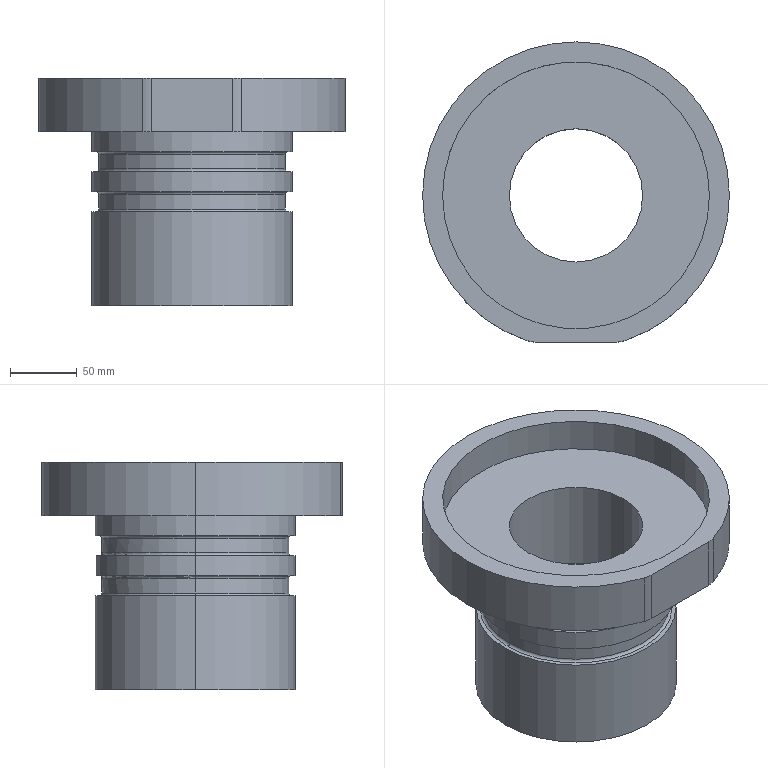Part | SolidWorks | features BaseBody 1 | 1 solid | 44 faces | box 230 x 225 x 170.5 mm | volume 1879136 mm3 | cylinder 19 | torus 12 | plane 11 | cone 2 | commonest cylinder face diameters 150 x7 140 x3 230 x3 40 x2 100 x2 200 x2
STEP:
#1=CARTESIAN_POINT('',(72.,-205.,70.5));
#2=VERTEX_POINT('',#1);
#3=CARTESIAN_POINT('',(-72.,-205.,70.5));
#4=VERTEX_POINT('',#3);
#5=CARTESIAN_POINT('',(0.,-205.,70.5));
#6=DIRECTION('',(0.,0.,-1.));
#7=DIRECTION('',(-1.,0.,0.));
#8=AXIS2_PLACEMENT_3D('',#5,#6,#7);
#9=CIRCLE('',#8,72.);
#10=EDGE_CURVE('',#2,#4,#9,.T.);
#11=ORIENTED_EDGE('',*,*,#10,.F.);
#12=CARTESIAN_POINT('',(70.,-205.,72.5));
#13=VERTEX_POINT('',#12);
#14=CARTESIAN_POINT('',(72.,-205.,72.5));
#15=DIRECTION('',(0.,1.,0.));
#16=DIRECTION('',(-1.,0.,0.));
#17=AXIS2_PLACEMENT_3D('',#14,#15,#16);
#18=CIRCLE('',#17,2.);
#19=EDGE_CURVE('',#2,#13,#18,.T.);
#20=ORIENTED_EDGE('',*,*,#19,.T.);
#21=CARTESIAN_POINT('',(-70.,-205.,72.5));
#22=VERTEX_POINT('',#21);
#23=CARTESIAN_POINT('',(0.,-205.,72.5));
#24=DIRECTION('',(0.,0.,1.));
#25=DIRECTION('',(-1.,0.,0.));
#26=AXIS2_PLACEMENT_3D('',#23,#24,#25);
#27=CIRCLE('',#26,70.);
#28=EDGE_CURVE('',#22,#13,#27,.T.);
#29=ORIENTED_EDGE('',*,*,#28,.F.);
#30=CARTESIAN_POINT('',(-72.,-205.,72.5));
#31=DIRECTION('',(0.,-1.,0.));
#32=DIRECTION('',(0.,0.,-1.));
#33=AXIS2_PLACEMENT_3D('',#30,#31,#32);
#34=CIRCLE('',#33,2.);
#35=EDGE_CURVE('',#4,#22,#34,.T.);
#36=ORIENTED_EDGE('',*,*,#35,.F.);
#37=EDGE_LOOP('',(#11,#20,#29,#36));
#38=FACE_OUTER_BOUND('',#37,.T.);
#39=CARTESIAN_POINT('',(0.,-205.,72.5));
#40=DIRECTION('',(0.,0.,-1.));
#41=DIRECTION('',(-1.,0.,0.));
#42=AXIS2_PLACEMENT_3D('',#39,#40,#41);
#43=TOROIDAL_SURFACE('',#42,72.,2.);
#44=ADVANCED_FACE('',(#38),#43,.F.);
#45=CARTESIAN_POINT('',(-72.,-205.,85.5));
#46=VERTEX_POINT('',#45);
#47=CARTESIAN_POINT('',(72.,-205.,85.5));
#48=VERTEX_POINT('',#47);
#49=CARTESIAN_POINT('',(0.,-205.,85.5));
#50=DIRECTION('',(0.,0.,1.));
#51=DIRECTION('',(1.,0.,0.));
#52=AXIS2_PLACEMENT_3D('',#49,#50,#51);
#53=CIRCLE('',#52,72.);
#54=EDGE_CURVE('',#46,#48,#53,.T.);
#55=ORIENTED_EDGE('',*,*,#54,.F.);
#56=CARTESIAN_POINT('',(-70.,-205.,83.5));
#57=VERTEX_POINT('',#56);
#58=CARTESIAN_POINT('',(-72.,-205.,83.5));
#59=DIRECTION('',(0.,1.,0.));
#60=DIRECTION('',(-1.,0.,0.));
#61=AXIS2_PLACEMENT_3D('',#58,#59,#60);
#62=CIRCLE('',#61,2.);
#63=EDGE_CURVE('',#46,#57,#62,.T.);
#64=ORIENTED_EDGE('',*,*,#63,.T.);
#65=CARTESIAN_POINT('',(70.,-205.,83.5));
#66=VERTEX_POINT('',#65);
#67=CARTESIAN_POINT('',(0.,-205.,83.5));
#68=DIRECTION('',(0.,0.,-1.));
#69=DIRECTION('',(1.,0.,0.));
#70=AXIS2_PLACEMENT_3D('',#67,#68,#69);
#71=CIRCLE('',#70,70.);
#72=EDGE_CURVE('',#66,#57,#71,.T.);
#73=ORIENTED_EDGE('',*,*,#72,.F.);
#74=CARTESIAN_POINT('',(72.,-205.,83.5));
#75=DIRECTION('',(0.,-1.,0.));
#76=DIRECTION('',(0.,0.,-1.));
#77=AXIS2_PLACEMENT_3D('',#74,#75,#76);
#78=CIRCLE('',#77,2.);
#79=EDGE_CURVE('',#48,#66,#78,.T.);
#80=ORIENTED_EDGE('',*,*,#79,.F.);
#81=EDGE_LOOP('',(#55,#64,#73,#80));
#82=FACE_OUTER_BOUND('',#81,.T.);
#83=CARTESIAN_POINT('',(0.,-205.,83.5));
#84=DIRECTION('',(0.,0.,1.));
#85=DIRECTION('',(1.,0.,0.));
#86=AXIS2_PLACEMENT_3D('',#83,#84,#85);
#87=TOROIDAL_SURFACE('',#86,72.,2.);
#88=ADVANCED_FACE('',(#82),#87,.F.);
#89=CARTESIAN_POINT('',(10.,-133.698,85.5));
#90=VERTEX_POINT('',#89);
#91=CARTESIAN_POINT('',(0.,-205.,85.5));
#92=DIRECTION('',(0.,0.,1.));
#93=DIRECTION('',(1.,0.,0.));
#94=AXIS2_PLACEMENT_3D('',#91,#92,#93);
#95=CIRCLE('',#94,72.);
#96=EDGE_CURVE('',#48,#90,#95,.T.);
#97=ORIENTED_EDGE('',*,*,#96,.F.);
#98=ORIENTED_EDGE('',*,*,#79,.T.);
#99=CARTESIAN_POINT('',(10.,-135.718,83.5));
#100=VERTEX_POINT('',#99);
#101=CARTESIAN_POINT('',(0.,-205.,83.5));
#102=DIRECTION('',(0.,0.,-1.));
#103=DIRECTION('',(1.,0.,0.));
#104=AXIS2_PLACEMENT_3D('',#101,#102,#103);
#105=CIRCLE('',#104,70.);
#106=EDGE_CURVE('',#100,#66,#105,.T.);
#107=ORIENTED_EDGE('',*,*,#106,.F.);
#108=CARTESIAN_POINT('',(10.,-135.718,83.5));
#109=CARTESIAN_POINT('',(10.,-135.718,83.763));
#110=CARTESIAN_POINT('',(10.,-135.664,84.03));
#111=CARTESIAN_POINT('',(10.,-135.46,84.513));
#112=CARTESIAN_POINT('',(10.,-135.308,84.735));
#113=CARTESIAN_POINT('',(10.,-135.028,85.011));
#114=CARTESIAN_POINT('',(10.,-134.925,85.094));
#115=CARTESIAN_POINT('',(10.,-134.704,85.239));
#116=CARTESIAN_POINT('',(10.,-134.588,85.3));
#117=CARTESIAN_POINT('',(10.,-134.345,85.399));
#118=CARTESIAN_POINT('',(10.,-134.217,85.437));
#119=CARTESIAN_POINT('',(10.,-133.96,85.487));
#120=CARTESIAN_POINT('',(10.,-133.83,85.5));
#121=CARTESIAN_POINT('',(10.,-133.698,85.5));
#122=B_SPLINE_CURVE_WITH_KNOTS('',3,(#108,#109,#110,#111,#112,#113,#114,#115,#116,#117,#118,#119,#120,#121),.UNSPECIFIED.,.F.,.F.,(4,2,2,2,2,2,4),(0.01202,0.01281,0.01359,0.01399,0.01438,0.01477,0.01516),.UNSPECIFIED.);
#123=EDGE_CURVE('',#100,#90,#122,.T.);
#124=ORIENTED_EDGE('',*,*,#123,.T.);
#125=EDGE_LOOP('',(#97,#98,#107,#124));
#126=FACE_OUTER_BOUND('',#125,.T.);
#127=CARTESIAN_POINT('',(0.,-205.,83.5));
#128=DIRECTION('',(0.,0.,1.));
#129=DIRECTION('',(1.,0.,0.));
#130=AXIS2_PLACEMENT_3D('',#127,#128,#129);
#131=TOROIDAL_SURFACE('',#130,72.,2.);
#132=ADVANCED_FACE('',(#126),#131,.F.);
#133=CARTESIAN_POINT('',(-115.,-205.,170.5));
#134=VERTEX_POINT('',#133);
#135=CARTESIAN_POINT('',(115.,-205.,170.5));
#136=VERTEX_POINT('',#135);
#137=CARTESIAN_POINT('',(0.,-205.,170.5));
#138=DIRECTION('',(0.,0.,-1.));
#139=DIRECTION('',(-1.,0.,0.));
#140=AXIS2_PLACEMENT_3D('',#137,#138,#139);
#141=CIRCLE('',#140,115.);
#142=EDGE_CURVE('',#134,#136,#141,.T.);
#143=ORIENTED_EDGE('',*,*,#142,.T.);
#144=CARTESIAN_POINT('',(115.,-205.,130.5));
#145=VERTEX_POINT('',#144);
#146=CARTESIAN_POINT('',(115.,-205.,170.5));
#147=DIRECTION('',(0.,0.,-1.));
#148=VECTOR('',#147,1000.);
#149=LINE('',#146,#148);
#150=EDGE_CURVE('',#136,#145,#149,.T.);
#151=ORIENTED_EDGE('',*,*,#150,.T.);
#152=CARTESIAN_POINT('',(-115.,-205.,130.5));
#153=VERTEX_POINT('',#152);
#154=CARTESIAN_POINT('',(0.,-205.,130.5));
#155=DIRECTION('',(0.,0.,-1.));
#156=DIRECTION('',(-1.,0.,0.));
#157=AXIS2_PLACEMENT_3D('',#154,#155,#156);
#158=CIRCLE('',#157,115.);
#159=EDGE_CURVE('',#153,#145,#158,.T.);
#160=ORIENTED_EDGE('',*,*,#159,.F.);
#161=CARTESIAN_POINT('',(-115.,-205.,170.5));
#162=DIRECTION('',(0.,0.,-1.));
#163=VECTOR('',#162,1000.);
#164=LINE('',#161,#163);
#165=EDGE_CURVE('',#134,#153,#164,.T.);
#166=ORIENTED_EDGE('',*,*,#165,.F.);
#167=EDGE_LOOP('',(#143,#151,#160,#166));
#168=FACE_OUTER_BOUND('',#167,.T.);
#169=CARTESIAN_POINT('',(0.,-205.,170.5));
#170=DIRECTION('',(0.,0.,-1.));
#171=DIRECTION('',(-1.,0.,0.));
#172=AXIS2_PLACEMENT_3D('',#169,#170,#171);
#173=CYLINDRICAL_SURFACE('',#172,115.);
#174=ADVANCED_FACE('',(#168),#173,.T.);
#175=CARTESIAN_POINT('',(-36.817,-313.947,170.5));
#176=VERTEX_POINT('',#175);
#177=CARTESIAN_POINT('',(0.,-205.,170.5));
#178=DIRECTION('',(0.,0.,-1.));
#179=DIRECTION('',(-1.,0.,0.));
#180=AXIS2_PLACEMENT_3D('',#177,#178,#179);
#181=CIRCLE('',#180,115.);
#182=EDGE_CURVE('',#176,#134,#181,.T.);
#183=ORIENTED_EDGE('',*,*,#182,.T.);
#184=ORIENTED_EDGE('',*,*,#165,.T.);
#185=CARTESIAN_POINT('',(-36.817,-313.947,130.5));
#186=VERTEX_POINT('',#185);
#187=CARTESIAN_POINT('',(0.,-205.,130.5));
#188=DIRECTION('',(0.,0.,-1.));
#189=DIRECTION('',(-1.,0.,0.));
#190=AXIS2_PLACEMENT_3D('',#187,#188,#189);
#191=CIRCLE('',#190,115.);
#192=EDGE_CURVE('',#186,#153,#191,.T.);
#193=ORIENTED_EDGE('',*,*,#192,.F.);
#194=CARTESIAN_POINT('',(-36.817,-313.947,170.5));
#195=DIRECTION('',(0.,0.,1.));
#196=VECTOR('',#195,1000.);
#197=LINE('',#194,#196);
#198=EDGE_CURVE('',#186,#176,#197,.T.);
#199=ORIENTED_EDGE('',*,*,#198,.T.);
#200=EDGE_LOOP('',(#183,#184,#193,#199));
#201=FACE_OUTER_BOUND('',#200,.T.);
#202=CARTESIAN_POINT('',(0.,-205.,170.5));
#203=DIRECTION('',(0.,0.,-1.));
#204=DIRECTION('',(-1.,0.,0.));
#205=AXIS2_PLACEMENT_3D('',#202,#203,#204);
#206=CYLINDRICAL_SURFACE('',#205,115.);
#207=ADVANCED_FACE('',(#201),#206,.T.);
#208=CARTESIAN_POINT('',(75.,-205.,130.5));
#209=VERTEX_POINT('',#208);
#210=CARTESIAN_POINT('',(-75.,-205.,130.5));
#211=VERTEX_POINT('',#210);
#212=CARTESIAN_POINT('',(0.,-205.,130.5));
#213=DIRECTION('',(0.,0.,1.));
#214=DIRECTION('',(-1.,0.,0.));
#215=AXIS2_PLACEMENT_3D('',#212,#213,#214);
#216=CIRCLE('',#215,75.);
#217=EDGE_CURVE('',#209,#211,#216,.T.);
#218=ORIENTED_EDGE('',*,*,#217,.F.);
#219=CARTESIAN_POINT('',(75.,-205.,115.5));
#220=VERTEX_POINT('',#219);
#221=CARTESIAN_POINT('',(75.,-205.,170.5));
#222=DIRECTION('',(0.,0.,-1.));
#223=VECTOR('',#222,1000.);
#224=LINE('',#221,#223);
#225=EDGE_CURVE('',#209,#220,#224,.T.);
#226=ORIENTED_EDGE('',*,*,#225,.T.);
#227=CARTESIAN_POINT('',(-75.,-205.,115.5));
#228=VERTEX_POINT('',#227);
#229=CARTESIAN_POINT('',(0.,-205.,115.5));
#230=DIRECTION('',(0.,0.,1.));
#231=DIRECTION('',(1.,0.,0.));
#232=AXIS2_PLACEMENT_3D('',#229,#230,#231);
#233=CIRCLE('',#232,75.);
#234=EDGE_CURVE('',#220,#228,#233,.T.);
#235=ORIENTED_EDGE('',*,*,#234,.T.);
#236=CARTESIAN_POINT('',(-75.,-205.,170.5));
#237=DIRECTION('',(0.,0.,-1.));
#238=VECTOR('',#237,1000.);
#239=LINE('',#236,#238);
#240=EDGE_CURVE('',#211,#228,#239,.T.);
#241=ORIENTED_EDGE('',*,*,#240,.F.);
#242=EDGE_LOOP('',(#218,#226,#235,#241));
#243=FACE_OUTER_BOUND('',#242,.T.);
#244=CARTESIAN_POINT('',(0.,-205.,170.5));
#245=DIRECTION('',(0.,0.,-1.));
#246=DIRECTION('',(-1.,0.,0.));
#247=AXIS2_PLACEMENT_3D('',#244,#245,#246);
#248=CYLINDRICAL_SURFACE('',#247,75.);
#249=ADVANCED_FACE('',(#243),#248,.T.);
#250=CARTESIAN_POINT('',(-70.,-205.,113.5));
#251=VERTEX_POINT('',#250);
#252=CARTESIAN_POINT('',(70.,-205.,113.5));
#253=VERTEX_POINT('',#252);
#254=CARTESIAN_POINT('',(0.,-205.,113.5));
#255=DIRECTION('',(0.,0.,-1.));
#256=DIRECTION('',(1.,0.,0.));
#257=AXIS2_PLACEMENT_3D('',#254,#255,#256);
#258=CIRCLE('',#257,70.);
#259=EDGE_CURVE('',#251,#253,#258,.T.);
#260=ORIENTED_EDGE('',*,*,#259,.T.);
#261=CARTESIAN_POINT('',(70.,-205.,102.5));
#262=VERTEX_POINT('',#261);
#263=CARTESIAN_POINT('',(70.,-205.,170.5));
#264=DIRECTION('',(0.,0.,-1.));
#265=VECTOR('',#264,1000.);
#266=LINE('',#263,#265);
#267=EDGE_CURVE('',#253,#262,#266,.T.);
#268=ORIENTED_EDGE('',*,*,#267,.T.);
#269=CARTESIAN_POINT('',(10.,-135.718,102.5));
#270=VERTEX_POINT('',#269);
#271=CARTESIAN_POINT('',(0.,-205.,102.5));
#272=DIRECTION('',(0.,0.,1.));
#273=DIRECTION('',(-1.,0.,0.));
#274=AXIS2_PLACEMENT_3D('',#271,#272,#273);
#275=CIRCLE('',#274,70.);
#276=EDGE_CURVE('',#262,#270,#275,.T.);
#277=ORIENTED_EDGE('',*,*,#276,.T.);
#278=CARTESIAN_POINT('',(10.,-135.718,170.5));
#279=DIRECTION('',(0.,0.,1.));
#280=VECTOR('',#279,1000.);
#281=LINE('',#278,#280);
#282=EDGE_CURVE('',#100,#270,#281,.T.);
#283=ORIENTED_EDGE('',*,*,#282,.F.);
#284=ORIENTED_EDGE('',*,*,#106,.T.);
#285=CARTESIAN_POINT('',(70.,-205.,170.5));
#286=DIRECTION('',(0.,0.,-1.));
#287=VECTOR('',#286,1000.);
#288=LINE('',#285,#287);
#289=EDGE_CURVE('',#66,#13,#288,.T.);
#290=ORIENTED_EDGE('',*,*,#289,.T.);
#291=CARTESIAN_POINT('',(0.,-205.,72.5));
#292=DIRECTION('',(0.,0.,1.));
#293=DIRECTION('',(-1.,0.,0.));
#294=AXIS2_PLACEMENT_3D('',#291,#292,#293);
#295=CIRCLE('',#294,70.);
#296=EDGE_CURVE('',#13,#22,#295,.T.);
#297=ORIENTED_EDGE('',*,*,#296,.T.);
#298=CARTESIAN_POINT('',(-70.,-205.,170.5));
#299=DIRECTION('',(0.,0.,-1.));
#300=VECTOR('',#299,1000.);
#301=LINE('',#298,#300);
#302=EDGE_CURVE('',#57,#22,#301,.T.);
#303=ORIENTED_EDGE('',*,*,#302,.F.);
#304=CARTESIAN_POINT('',(-10.,-135.718,83.5));
#305=VERTEX_POINT('',#304);
#306=CARTESIAN_POINT('',(0.,-205.,83.5));
#307=DIRECTION('',(0.,0.,-1.));
#308=DIRECTION('',(1.,0.,0.));
#309=AXIS2_PLACEMENT_3D('',#306,#307,#308);
#310=CIRCLE('',#309,70.);
#311=EDGE_CURVE('',#57,#305,#310,.T.);
#312=ORIENTED_EDGE('',*,*,#311,.T.);
#313=CARTESIAN_POINT('',(-10.,-135.718,102.5));
#314=VERTEX_POINT('',#313);
#315=CARTESIAN_POINT('',(-10.,-135.718,170.5));
#316=DIRECTION('',(0.,0.,-1.));
#317=VECTOR('',#316,1000.);
#318=LINE('',#315,#317);
#319=EDGE_CURVE('',#314,#305,#318,.T.);
#320=ORIENTED_EDGE('',*,*,#319,.F.);
#321=CARTESIAN_POINT('',(-70.,-205.,102.5));
#322=VERTEX_POINT('',#321);
#323=CARTESIAN_POINT('',(0.,-205.,102.5));
#324=DIRECTION('',(0.,0.,1.));
#325=DIRECTION('',(-1.,0.,0.));
#326=AXIS2_PLACEMENT_3D('',#323,#324,#325);
#327=CIRCLE('',#326,70.);
#328=EDGE_CURVE('',#314,#322,#327,.T.);
#329=ORIENTED_EDGE('',*,*,#328,.T.);
#330=CARTESIAN_POINT('',(-70.,-205.,170.5));
#331=DIRECTION('',(0.,0.,-1.));
#332=VECTOR('',#331,1000.);
#333=LINE('',#330,#332);
#334=EDGE_CURVE('',#251,#322,#333,.T.);
#335=ORIENTED_EDGE('',*,*,#334,.F.);
#336=EDGE_LOOP('',(#260,#268,#277,#283,#284,#290,#297,#303,#312,#320,#329,#335));
#337=FACE_OUTER_BOUND('',#336,.T.);
#338=CARTESIAN_POINT('',(0.,-205.,170.5));
#339=DIRECTION('',(0.,0.,-1.));
#340=DIRECTION('',(-1.,0.,0.));
#341=AXIS2_PLACEMENT_3D('',#338,#339,#340);
#342=CYLINDRICAL_SURFACE('',#341,70.);
#343=ADVANCED_FACE('',(#337),#342,.T.);
#344=ORIENTED_EDGE('',*,*,#267,.F.);
#345=CARTESIAN_POINT('',(0.,-205.,113.5));
#346=DIRECTION('',(0.,0.,-1.));
#347=DIRECTION('',(1.,0.,0.));
#348=AXIS2_PLACEMENT_3D('',#345,#346,#347);
#349=CIRCLE('',#348,70.);
#350=EDGE_CURVE('',#253,#251,#349,.T.);
#351=ORIENTED_EDGE('',*,*,#350,.T.);
#352=ORIENTED_EDGE('',*,*,#334,.T.);
#353=CARTESIAN_POINT('',(0.,-205.,102.5));
#354=DIRECTION('',(0.,0.,1.));
#355=DIRECTION('',(-1.,0.,0.));
#356=AXIS2_PLACEMENT_3D('',#353,#354,#355);
#357=CIRCLE('',#356,70.);
#358=EDGE_CURVE('',#322,#262,#357,.T.);
#359=ORIENTED_EDGE('',*,*,#358,.T.);
#360=EDGE_LOOP('',(#344,#351,#352,#359));
#361=FACE_OUTER_BOUND('',#360,.T.);
#362=CARTESIAN_POINT('',(0.,-205.,170.5));
#363=DIRECTION('',(0.,0.,-1.));
#364=DIRECTION('',(-1.,0.,0.));
#365=AXIS2_PLACEMENT_3D('',#362,#363,#364);
#366=CYLINDRICAL_SURFACE('',#365,70.);
#367=ADVANCED_FACE('',(#361),#366,.T.);
#368=CARTESIAN_POINT('',(72.,-205.,100.5));
#369=VERTEX_POINT('',#368);
#370=CARTESIAN_POINT('',(-72.,-205.,100.5));
#371=VERTEX_POINT('',#370);
#372=CARTESIAN_POINT('',(0.,-205.,100.5));
#373=DIRECTION('',(0.,0.,-1.));
#374=DIRECTION('',(-1.,0.,0.));
#375=AXIS2_PLACEMENT_3D('',#372,#373,#374);
#376=CIRCLE('',#375,72.);
#377=EDGE_CURVE('',#369,#371,#376,.T.);
#378=ORIENTED_EDGE('',*,*,#377,.F.);
#379=CARTESIAN_POINT('',(72.,-205.,102.5));
#380=DIRECTION('',(0.,1.,0.));
#381=DIRECTION('',(-1.,0.,0.));
#382=AXIS2_PLACEMENT_3D('',#379,#380,#381);
#383=CIRCLE('',#382,2.);
#384=EDGE_CURVE('',#369,#262,#383,.T.);
#385=ORIENTED_EDGE('',*,*,#384,.T.);
#386=ORIENTED_EDGE('',*,*,#358,.F.);
#387=CARTESIAN_POINT('',(-72.,-205.,102.5));
#388=DIRECTION('',(0.,-1.,0.));
#389=DIRECTION('',(0.,0.,-1.));
#390=AXIS2_PLACEMENT_3D('',#387,#388,#389);
#391=CIRCLE('',#390,2.);
#392=EDGE_CURVE('',#371,#322,#391,.T.);
#393=ORIENTED_EDGE('',*,*,#392,.F.);
#394=EDGE_LOOP('',(#378,#385,#386,#393));
#395=FACE_OUTER_BOUND('',#394,.T.);
#396=CARTESIAN_POINT('',(0.,-205.,102.5));
#397=DIRECTION('',(0.,0.,-1.));
#398=DIRECTION('',(-1.,0.,0.));
#399=AXIS2_PLACEMENT_3D('',#396,#397,#398);
#400=TOROIDAL_SURFACE('',#399,72.,2.);
#401=ADVANCED_FACE('',(#395),#400,.F.);
#402=CARTESIAN_POINT('',(-10.,-133.698,100.5));
#403=VERTEX_POINT('',#402);
#404=CARTESIAN_POINT('',(0.,-205.,100.5));
#405=DIRECTION('',(0.,0.,-1.));
#406=DIRECTION('',(-1.,0.,0.));
#407=AXIS2_PLACEMENT_3D('',#404,#405,#406);
#408=CIRCLE('',#407,72.);
#409=EDGE_CURVE('',#371,#403,#408,.T.);
#410=ORIENTED_EDGE('',*,*,#409,.F.);
#411=ORIENTED_EDGE('',*,*,#392,.T.);
#412=ORIENTED_EDGE('',*,*,#328,.F.);
#413=CARTESIAN_POINT('',(-10.,-135.718,102.5));
#414=CARTESIAN_POINT('',(-10.,-135.718,102.369));
#415=CARTESIAN_POINT('',(-10.,-135.705,102.237));
#416=CARTESIAN_POINT('',(-10.,-135.653,101.978));
#417=CARTESIAN_POINT('',(-10.,-135.614,101.853));
#418=CARTESIAN_POINT('',(-10.,-135.462,101.49));
#419=CARTESIAN_POINT('',(-10.,-135.308,101.265));
#420=CARTESIAN_POINT('',(-10.,-135.028,100.989));
#421=CARTESIAN_POINT('',(-10.,-134.926,100.907));
#422=CARTESIAN_POINT('',(-10.,-134.706,100.762));
#423=CARTESIAN_POINT('',(-10.,-134.588,100.7));
#424=CARTESIAN_POINT('',(-10.,-134.224,100.552));
#425=CARTESIAN_POINT('',(-10.,-133.96,100.5));
#426=CARTESIAN_POINT('',(-10.,-133.698,100.5));
#427=B_SPLINE_CURVE_WITH_KNOTS('',3,(#413,#414,#415,#416,#417,#418,#419,#420,#421,#422,#423,#424,#425,#426),.UNSPECIFIED.,.F.,.F.,(4,2,2,2,2,2,4),(0.01118,0.01157,0.01196,0.01275,0.01314,0.01353,0.01432),.UNSPECIFIED.);
#428=EDGE_CURVE('',#314,#403,#427,.T.);
#429=ORIENTED_EDGE('',*,*,#428,.T.);
#430=EDGE_LOOP('',(#410,#411,#412,#429));
#431=FACE_OUTER_BOUND('',#430,.T.);
#432=CARTESIAN_POINT('',(0.,-205.,102.5));
#433=DIRECTION('',(0.,0.,-1.));
#434=DIRECTION('',(-1.,0.,0.));
#435=AXIS2_PLACEMENT_3D('',#432,#433,#434);
#436=TOROIDAL_SURFACE('',#435,72.,2.);
#437=ADVANCED_FACE('',(#431),#436,.F.);
#438=CARTESIAN_POINT('',(-72.,-205.,115.5));
#439=VERTEX_POINT('',#438);
#440=CARTESIAN_POINT('',(72.,-205.,115.5));
#441=VERTEX_POINT('',#440);
#442=CARTESIAN_POINT('',(0.,-205.,115.5));
#443=DIRECTION('',(0.,0.,1.));
#444=DIRECTION('',(1.,0.,0.));
#445=AXIS2_PLACEMENT_3D('',#442,#443,#444);
#446=CIRCLE('',#445,72.);
#447=EDGE_CURVE('',#439,#441,#446,.T.);
#448=ORIENTED_EDGE('',*,*,#447,.F.);
#449=CARTESIAN_POINT('',(-72.,-205.,113.5));
#450=DIRECTION('',(0.,1.,0.));
#451=DIRECTION('',(-1.,0.,0.));
#452=AXIS2_PLACEMENT_3D('',#449,#450,#451);
#453=CIRCLE('',#452,2.);
#454=EDGE_CURVE('',#439,#251,#453,.T.);
#455=ORIENTED_EDGE('',*,*,#454,.T.);
#456=ORIENTED_EDGE('',*,*,#350,.F.);
#457=CARTESIAN_POINT('',(72.,-205.,113.5));
#458=DIRECTION('',(0.,-1.,0.));
#459=DIRECTION('',(0.,0.,-1.));
#460=AXIS2_PLACEMENT_3D('',#457,#458,#459);
#461=CIRCLE('',#460,2.);
#462=EDGE_CURVE('',#441,#253,#461,.T.);
#463=ORIENTED_EDGE('',*,*,#462,.F.);
#464=EDGE_LOOP('',(#448,#455,#456,#463));
#465=FACE_OUTER_BOUND('',#464,.T.);
#466=CARTESIAN_POINT('',(0.,-205.,113.5));
#467=DIRECTION('',(0.,0.,1.));
#468=DIRECTION('',(1.,0.,0.));
#469=AXIS2_PLACEMENT_3D('',#466,#467,#468);
#470=TOROIDAL_SURFACE('',#469,72.,2.);
#471=ADVANCED_FACE('',(#465),#470,.F.);
#472=CARTESIAN_POINT('',(-50.,-205.,145.5));
#473=VERTEX_POINT('',#472);
#474=CARTESIAN_POINT('',(50.,-205.,145.5));
#475=VERTEX_POINT('',#474);
#476=CARTESIAN_POINT('',(0.,-205.,145.5));
#477=DIRECTION('',(0.,0.,1.));
#478=DIRECTION('',(-1.,0.,0.));
#479=AXIS2_PLACEMENT_3D('',#476,#477,#478);
#480=CIRCLE('',#479,50.);
#481=EDGE_CURVE('',#473,#475,#480,.T.);
#482=ORIENTED_EDGE('',*,*,#481,.T.);
#483=CARTESIAN_POINT('',(50.,-205.,75.5));
#484=VERTEX_POINT('',#483);
#485=CARTESIAN_POINT('',(50.,-205.,170.5));
#486=DIRECTION('',(0.,0.,-1.));
#487=VECTOR('',#486,1000.);
#488=LINE('',#485,#487);
#489=EDGE_CURVE('',#475,#484,#488,.T.);
#490=ORIENTED_EDGE('',*,*,#489,.T.);
#491=CARTESIAN_POINT('',(-50.,-205.,75.5));
#492=VERTEX_POINT('',#491);
#493=CARTESIAN_POINT('',(0.,-205.,75.5));
#494=DIRECTION('',(0.,0.,-1.));
#495=DIRECTION('',(1.,0.,0.));
#496=AXIS2_PLACEMENT_3D('',#493,#494,#495);
#497=CIRCLE('',#496,50.);
#498=EDGE_CURVE('',#484,#492,#497,.T.);
#499=ORIENTED_EDGE('',*,*,#498,.T.);
#500=CARTESIAN_POINT('',(-50.,-205.,170.5));
#501=DIRECTION('',(0.,0.,-1.));
#502=VECTOR('',#501,1000.);
#503=LINE('',#500,#502);
#504=EDGE_CURVE('',#473,#492,#503,.T.);
#505=ORIENTED_EDGE('',*,*,#504,.F.);
#506=EDGE_LOOP('',(#482,#490,#499,#505));
#507=FACE_OUTER_BOUND('',#506,.T.);
#508=CARTESIAN_POINT('',(0.,-205.,170.5));
#509=DIRECTION('',(0.,0.,-1.));
#510=DIRECTION('',(-1.,0.,0.));
#511=AXIS2_PLACEMENT_3D('',#508,#509,#510);
#512=CYLINDRICAL_SURFACE('',#511,50.);
#513=ADVANCED_FACE('',(#507),#512,.F.);
#514=CARTESIAN_POINT('',(0.,-205.,75.5));
#515=DIRECTION('',(0.,0.,-1.));
#516=DIRECTION('',(1.,0.,0.));
#517=AXIS2_PLACEMENT_3D('',#514,#515,#516);
#518=CIRCLE('',#517,50.);
#519=EDGE_CURVE('',#492,#484,#518,.T.);
#520=ORIENTED_EDGE('',*,*,#519,.F.);
#521=CARTESIAN_POINT('',(-56.206,-205.,4.564));
#522=VERTEX_POINT('',#521);
#523=CARTESIAN_POINT('',(-50.,-205.,75.5));
#524=DIRECTION('',(-0.08716,0.,-0.9962));
#525=VECTOR('',#524,1000.);
#526=LINE('',#523,#525);
#527=EDGE_CURVE('',#492,#522,#526,.T.);
#528=ORIENTED_EDGE('',*,*,#527,.T.);
#529=CARTESIAN_POINT('',(56.206,-205.,4.564));
#530=VERTEX_POINT('',#529);
#531=CARTESIAN_POINT('',(0.,-205.,4.564));
#532=DIRECTION('',(0.,0.,-1.));
#533=DIRECTION('',(1.,0.,0.));
#534=AXIS2_PLACEMENT_3D('',#531,#532,#533);
#535=CIRCLE('',#534,56.206);
#536=EDGE_CURVE('',#522,#530,#535,.T.);
#537=ORIENTED_EDGE('',*,*,#536,.T.);
#538=CARTESIAN_POINT('',(50.,-205.,75.5));
#539=DIRECTION('',(0.08716,0.,-0.9962));
#540=VECTOR('',#539,1000.);
#541=LINE('',#538,#540);
#542=EDGE_CURVE('',#484,#530,#541,.T.);
#543=ORIENTED_EDGE('',*,*,#542,.F.);
#544=EDGE_LOOP('',(#520,#528,#537,#543));
#545=FACE_OUTER_BOUND('',#544,.T.);
#546=CARTESIAN_POINT('',(0.,-205.,75.5));
#547=DIRECTION('',(0.,0.,-1.));
#548=DIRECTION('',(1.,0.,0.));
#549=AXIS2_PLACEMENT_3D('',#546,#547,#548);
#550=CONICAL_SURFACE('',#549,50.,0.08727);
#551=ADVANCED_FACE('',(#545),#550,.F.);
#552=ORIENTED_EDGE('',*,*,#536,.F.);
#553=CARTESIAN_POINT('',(-61.187,-205.,0.));
#554=VERTEX_POINT('',#553);
#555=CARTESIAN_POINT('',(-61.187,-205.,5.));
#556=DIRECTION('',(0.,1.,0.));
#557=DIRECTION('',(-1.,0.,0.));
#558=AXIS2_PLACEMENT_3D('',#555,#556,#557);
#559=CIRCLE('',#558,5.);
#560=EDGE_CURVE('',#522,#554,#559,.T.);
#561=ORIENTED_EDGE('',*,*,#560,.T.);
#562=CARTESIAN_POINT('',(61.187,-205.,0.));
#563=VERTEX_POINT('',#562);
#564=CARTESIAN_POINT('',(0.,-205.,0.));
#565=DIRECTION('',(0.,0.,1.));
#566=DIRECTION('',(1.,0.,0.));
#567=AXIS2_PLACEMENT_3D('',#564,#565,#566);
#568=CIRCLE('',#567,61.187);
#569=EDGE_CURVE('',#563,#554,#568,.T.);
#570=ORIENTED_EDGE('',*,*,#569,.F.);
#571=CARTESIAN_POINT('',(61.187,-205.,5.));
#572=DIRECTION('',(0.,-1.,0.));
#573=DIRECTION('',(0.,0.,-1.));
#574=AXIS2_PLACEMENT_3D('',#571,#572,#573);
#575=CIRCLE('',#574,5.);
#576=EDGE_CURVE('',#530,#563,#575,.T.);
#577=ORIENTED_EDGE('',*,*,#576,.F.);
#578=EDGE_LOOP('',(#552,#561,#570,#577));
#579=FACE_OUTER_BOUND('',#578,.T.);
#580=CARTESIAN_POINT('',(0.,-205.,5.));
#581=DIRECTION('',(0.,0.,1.));
#582=DIRECTION('',(1.,0.,0.));
#583=AXIS2_PLACEMENT_3D('',#580,#581,#582);
#584=TOROIDAL_SURFACE('',#583,61.187,5.);
#585=ADVANCED_FACE('',(#579),#584,.T.);
#586=CARTESIAN_POINT('',(100.,-205.,170.5));
#587=VERTEX_POINT('',#586);
#588=CARTESIAN_POINT('',(-100.,-205.,170.5));
#589=VERTEX_POINT('',#588);
#590=CARTESIAN_POINT('',(0.,-205.,170.5));
#591=DIRECTION('',(0.,0.,-1.));
#592=DIRECTION('',(-1.,0.,0.));
#593=AXIS2_PLACEMENT_3D('',#590,#591,#592);
#594=CIRCLE('',#593,100.);
#595=EDGE_CURVE('',#587,#589,#594,.T.);
#596=ORIENTED_EDGE('',*,*,#595,.F.);
#597=CARTESIAN_POINT('',(100.,-205.,145.5));
#598=VERTEX_POINT('',#597);
#599=CARTESIAN_POINT('',(100.,-205.,170.5));
#600=DIRECTION('',(0.,0.,-1.));
#601=VECTOR('',#600,1000.);
#602=LINE('',#599,#601);
#603=EDGE_CURVE('',#587,#598,#602,.T.);
#604=ORIENTED_EDGE('',*,*,#603,.T.);
#605=CARTESIAN_POINT('',(-100.,-205.,145.5));
#606=VERTEX_POINT('',#605);
#607=CARTESIAN_POINT('',(0.,-205.,145.5));
#608=DIRECTION('',(0.,0.,-1.));
#609=DIRECTION('',(-1.,0.,0.));
#610=AXIS2_PLACEMENT_3D('',#607,#608,#609);
#611=CIRCLE('',#610,100.);
#612=EDGE_CURVE('',#598,#606,#611,.T.);
#613=ORIENTED_EDGE('',*,*,#612,.T.);
#614=CARTESIAN_POINT('',(-100.,-205.,170.5));
#615=DIRECTION('',(0.,0.,-1.));
#616=VECTOR('',#615,1000.);
#617=LINE('',#614,#616);
#618=EDGE_CURVE('',#589,#606,#617,.T.);
#619=ORIENTED_EDGE('',*,*,#618,.F.);
#620=EDGE_LOOP('',(#596,#604,#613,#619));
#621=FACE_OUTER_BOUND('',#620,.T.);
#622=CARTESIAN_POINT('',(0.,-205.,170.5));
#623=DIRECTION('',(0.,0.,-1.));
#624=DIRECTION('',(-1.,0.,0.));
#625=AXIS2_PLACEMENT_3D('',#622,#623,#624);
#626=CYLINDRICAL_SURFACE('',#625,100.);
#627=ADVANCED_FACE('',(#621),#626,.F.);
#628=CARTESIAN_POINT('',(10.,-130.67,100.5));
#629=VERTEX_POINT('',#628);
#630=CARTESIAN_POINT('',(75.,-205.,100.5));
#631=VERTEX_POINT('',#630);
#632=CARTESIAN_POINT('',(0.,-205.,100.5));
#633=DIRECTION('',(0.,0.,-1.));
#634=DIRECTION('',(-1.,0.,0.));
#635=AXIS2_PLACEMENT_3D('',#632,#633,#634);
#636=CIRCLE('',#635,75.);
#637=EDGE_CURVE('',#629,#631,#636,.T.);
#638=ORIENTED_EDGE('',*,*,#637,.T.);
#639=CARTESIAN_POINT('',(75.,-205.,85.5));
#640=VERTEX_POINT('',#639);
#641=CARTESIAN_POINT('',(75.,-205.,170.5));
#642=DIRECTION('',(0.,0.,-1.));
#643=VECTOR('',#642,1000.);
#644=LINE('',#641,#643);
#645=EDGE_CURVE('',#631,#640,#644,.T.);
#646=ORIENTED_EDGE('',*,*,#645,.T.);
#647=CARTESIAN_POINT('',(10.,-130.67,85.5));
#648=VERTEX_POINT('',#647);
#649=CARTESIAN_POINT('',(0.,-205.,85.5));
#650=DIRECTION('',(0.,0.,1.));
#651=DIRECTION('',(1.,0.,0.));
#652=AXIS2_PLACEMENT_3D('',#649,#650,#651);
#653=CIRCLE('',#652,75.);
#654=EDGE_CURVE('',#640,#648,#653,.T.);
#655=ORIENTED_EDGE('',*,*,#654,.T.);
#656=CARTESIAN_POINT('',(10.,-130.67,170.5));
#657=DIRECTION('',(0.,0.,1.));
#658=VECTOR('',#657,1000.);
#659=LINE('',#656,#658);
#660=EDGE_CURVE('',#648,#629,#659,.T.);
#661=ORIENTED_EDGE('',*,*,#660,.T.);
#662=EDGE_LOOP('',(#638,#646,#655,#661));
#663=FACE_OUTER_BOUND('',#662,.T.);
#664=CARTESIAN_POINT('',(0.,-205.,170.5));
#665=DIRECTION('',(0.,0.,-1.));
#666=DIRECTION('',(-1.,0.,0.));
#667=AXIS2_PLACEMENT_3D('',#664,#665,#666);
#668=CYLINDRICAL_SURFACE('',#667,75.);
#669=ADVANCED_FACE('',(#663),#668,.T.);
#670=ORIENTED_EDGE('',*,*,#645,.F.);
#671=CARTESIAN_POINT('',(-75.,-205.,100.5));
#672=VERTEX_POINT('',#671);
#673=CARTESIAN_POINT('',(0.,-205.,100.5));
#674=DIRECTION('',(0.,0.,-1.));
#675=DIRECTION('',(-1.,0.,0.));
#676=AXIS2_PLACEMENT_3D('',#673,#674,#675);
#677=CIRCLE('',#676,75.);
#678=EDGE_CURVE('',#631,#672,#677,.T.);
#679=ORIENTED_EDGE('',*,*,#678,.T.);
#680=CARTESIAN_POINT('',(-75.,-205.,85.5));
#681=VERTEX_POINT('',#680);
#682=CARTESIAN_POINT('',(-75.,-205.,170.5));
#683=DIRECTION('',(0.,0.,-1.));
#684=VECTOR('',#683,1000.);
#685=LINE('',#682,#684);
#686=EDGE_CURVE('',#672,#681,#685,.T.);
#687=ORIENTED_EDGE('',*,*,#686,.T.);
#688=CARTESIAN_POINT('',(0.,-205.,85.5));
#689=DIRECTION('',(0.,0.,1.));
#690=DIRECTION('',(1.,0.,0.));
#691=AXIS2_PLACEMENT_3D('',#688,#689,#690);
#692=CIRCLE('',#691,75.);
#693=EDGE_CURVE('',#681,#640,#692,.T.);
#694=ORIENTED_EDGE('',*,*,#693,.T.);
#695=EDGE_LOOP('',(#670,#679,#687,#694));
#696=FACE_OUTER_BOUND('',#695,.T.);
#697=CARTESIAN_POINT('',(0.,-205.,170.5));
#698=DIRECTION('',(0.,0.,-1.));
#699=DIRECTION('',(-1.,0.,0.));
#700=AXIS2_PLACEMENT_3D('',#697,#698,#699);
#701=CYLINDRICAL_SURFACE('',#700,75.);
#702=ADVANCED_FACE('',(#696),#701,.T.);
#703=CARTESIAN_POINT('',(-75.,-205.,70.5));
#704=VERTEX_POINT('',#703);
#705=CARTESIAN_POINT('',(75.,-205.,70.5));
#706=VERTEX_POINT('',#705);
#707=CARTESIAN_POINT('',(0.,-205.,70.5));
#708=DIRECTION('',(0.,0.,-1.));
#709=DIRECTION('',(-1.,0.,0.));
#710=AXIS2_PLACEMENT_3D('',#707,#708,#709);
#711=CIRCLE('',#710,75.);
#712=EDGE_CURVE('',#704,#706,#711,.T.);
#713=ORIENTED_EDGE('',*,*,#712,.T.);
#714=CARTESIAN_POINT('',(75.,-205.,0.));
#715=VERTEX_POINT('',#714);
#716=CARTESIAN_POINT('',(75.,-205.,170.5));
#717=DIRECTION('',(0.,0.,-1.));
#718=VECTOR('',#717,1000.);
#719=LINE('',#716,#718);
#720=EDGE_CURVE('',#706,#715,#719,.T.);
#721=ORIENTED_EDGE('',*,*,#720,.T.);
#722=CARTESIAN_POINT('',(-75.,-205.,0.));
#723=VERTEX_POINT('',#722);
#724=CARTESIAN_POINT('',(0.,-205.,0.));
#725=DIRECTION('',(0.,0.,1.));
#726=DIRECTION('',(1.,0.,0.));
#727=AXIS2_PLACEMENT_3D('',#724,#725,#726);
#728=CIRCLE('',#727,75.);
#729=EDGE_CURVE('',#715,#723,#728,.T.);
#730=ORIENTED_EDGE('',*,*,#729,.T.);
#731=CARTESIAN_POINT('',(-75.,-205.,170.5));
#732=DIRECTION('',(0.,0.,-1.));
#733=VECTOR('',#732,1000.);
#734=LINE('',#731,#733);
#735=EDGE_CURVE('',#704,#723,#734,.T.);
#736=ORIENTED_EDGE('',*,*,#735,.F.);
#737=EDGE_LOOP('',(#713,#721,#730,#736));
#738=FACE_OUTER_BOUND('',#737,.T.);
#739=CARTESIAN_POINT('',(0.,-205.,170.5));
#740=DIRECTION('',(0.,0.,-1.));
#741=DIRECTION('',(-1.,0.,0.));
#742=AXIS2_PLACEMENT_3D('',#739,#740,#741);
#743=CYLINDRICAL_SURFACE('',#742,75.);
#744=ADVANCED_FACE('',(#738),#743,.T.);
#745=ORIENTED_EDGE('',*,*,#720,.F.);
#746=CARTESIAN_POINT('',(0.,-205.,70.5));
#747=DIRECTION('',(0.,0.,-1.));
#748=DIRECTION('',(-1.,0.,0.));
#749=AXIS2_PLACEMENT_3D('',#746,#747,#748);
#750=CIRCLE('',#749,75.);
#751=EDGE_CURVE('',#706,#704,#750,.T.);
#752=ORIENTED_EDGE('',*,*,#751,.T.);
#753=ORIENTED_EDGE('',*,*,#735,.T.);
#754=CARTESIAN_POINT('',(0.,-205.,0.));
#755=DIRECTION('',(0.,0.,1.));
#756=DIRECTION('',(1.,0.,0.));
#757=AXIS2_PLACEMENT_3D('',#754,#755,#756);
#758=CIRCLE('',#757,75.);
#759=EDGE_CURVE('',#723,#715,#758,.T.);
#760=ORIENTED_EDGE('',*,*,#759,.T.);
#761=EDGE_LOOP('',(#745,#752,#753,#760));
#762=FACE_OUTER_BOUND('',#761,.T.);
#763=CARTESIAN_POINT('',(0.,-205.,170.5));
#764=DIRECTION('',(0.,0.,-1.));
#765=DIRECTION('',(-1.,0.,0.));
#766=AXIS2_PLACEMENT_3D('',#763,#764,#765);
#767=CYLINDRICAL_SURFACE('',#766,75.);
#768=ADVANCED_FACE('',(#762),#767,.T.);
#769=ORIENTED_EDGE('',*,*,#686,.F.);
#770=CARTESIAN_POINT('',(-10.,-130.67,100.5));
#771=VERTEX_POINT('',#770);
#772=CARTESIAN_POINT('',(0.,-205.,100.5));
#773=DIRECTION('',(0.,0.,-1.));
#774=DIRECTION('',(-1.,0.,0.));
#775=AXIS2_PLACEMENT_3D('',#772,#773,#774);
#776=CIRCLE('',#775,75.);
#777=EDGE_CURVE('',#672,#771,#776,.T.);
#778=ORIENTED_EDGE('',*,*,#777,.T.);
#779=CARTESIAN_POINT('',(-10.,-130.67,85.5));
#780=VERTEX_POINT('',#779);
#781=CARTESIAN_POINT('',(-10.,-130.67,170.5));
#782=DIRECTION('',(0.,0.,-1.));
#783=VECTOR('',#782,1000.);
#784=LINE('',#781,#783);
#785=EDGE_CURVE('',#771,#780,#784,.T.);
#786=ORIENTED_EDGE('',*,*,#785,.T.);
#787=CARTESIAN_POINT('',(0.,-205.,85.5));
#788=DIRECTION('',(0.,0.,1.));
#789=DIRECTION('',(1.,0.,0.));
#790=AXIS2_PLACEMENT_3D('',#787,#788,#789);
#791=CIRCLE('',#790,75.);
#792=EDGE_CURVE('',#780,#681,#791,.T.);
#793=ORIENTED_EDGE('',*,*,#792,.T.);
#794=EDGE_LOOP('',(#769,#778,#786,#793));
#795=FACE_OUTER_BOUND('',#794,.T.);
#796=CARTESIAN_POINT('',(0.,-205.,170.5));
#797=DIRECTION('',(0.,0.,-1.));
#798=DIRECTION('',(-1.,0.,0.));
#799=AXIS2_PLACEMENT_3D('',#796,#797,#798);
#800=CYLINDRICAL_SURFACE('',#799,75.);
#801=ADVANCED_FACE('',(#795),#800,.T.);
#802=ORIENTED_EDGE('',*,*,#603,.F.);
#803=CARTESIAN_POINT('',(0.,-205.,170.5));
#804=DIRECTION('',(0.,0.,-1.));
#805=DIRECTION('',(-1.,0.,0.));
#806=AXIS2_PLACEMENT_3D('',#803,#804,#805);
#807=CIRCLE('',#806,100.);
#808=EDGE_CURVE('',#589,#587,#807,.T.);
#809=ORIENTED_EDGE('',*,*,#808,.F.);
#810=ORIENTED_EDGE('',*,*,#618,.T.);
#811=CARTESIAN_POINT('',(0.,-205.,145.5));
#812=DIRECTION('',(0.,0.,-1.));
#813=DIRECTION('',(-1.,0.,0.));
#814=AXIS2_PLACEMENT_3D('',#811,#812,#813);
#815=CIRCLE('',#814,100.);
#816=EDGE_CURVE('',#606,#598,#815,.T.);
#817=ORIENTED_EDGE('',*,*,#816,.T.);
#818=EDGE_LOOP('',(#802,#809,#810,#817));
#819=FACE_OUTER_BOUND('',#818,.T.);
#820=CARTESIAN_POINT('',(0.,-205.,170.5));
#821=DIRECTION('',(0.,0.,-1.));
#822=DIRECTION('',(-1.,0.,0.));
#823=AXIS2_PLACEMENT_3D('',#820,#821,#822);
#824=CYLINDRICAL_SURFACE('',#823,100.);
#825=ADVANCED_FACE('',(#819),#824,.F.);
#826=ORIENTED_EDGE('',*,*,#481,.F.);
#827=CARTESIAN_POINT('',(0.,-205.,145.5));
#828=DIRECTION('',(0.,0.,1.));
#829=DIRECTION('',(-1.,0.,0.));
#830=AXIS2_PLACEMENT_3D('',#827,#828,#829);
#831=CIRCLE('',#830,50.);
#832=EDGE_CURVE('',#475,#473,#831,.T.);
#833=ORIENTED_EDGE('',*,*,#832,.F.);
#834=EDGE_LOOP('',(#826,#833));
#835=FACE_BOUND('',#834,.T.);
#836=ORIENTED_EDGE('',*,*,#816,.F.);
#837=ORIENTED_EDGE('',*,*,#612,.F.);
#838=EDGE_LOOP('',(#836,#837));
#839=FACE_OUTER_BOUND('',#838,.T.);
#840=CARTESIAN_POINT('',(0.,-205.,145.5));
#841=DIRECTION('',(0.,0.,-1.));
#842=DIRECTION('',(-1.,0.,0.));
#843=AXIS2_PLACEMENT_3D('',#840,#841,#842);
#844=PLANE('',#843);
#845=ADVANCED_FACE('',(#835,#839),#844,.F.);
#846=ORIENTED_EDGE('',*,*,#560,.F.);
#847=CARTESIAN_POINT('',(0.,-205.,4.564));
#848=DIRECTION('',(0.,0.,-1.));
#849=DIRECTION('',(1.,0.,0.));
#850=AXIS2_PLACEMENT_3D('',#847,#848,#849);
#851=CIRCLE('',#850,56.206);
#852=EDGE_CURVE('',#530,#522,#851,.T.);
#853=ORIENTED_EDGE('',*,*,#852,.F.);
#854=ORIENTED_EDGE('',*,*,#576,.T.);
#855=CARTESIAN_POINT('',(0.,-205.,0.));
#856=DIRECTION('',(0.,0.,1.));
#857=DIRECTION('',(1.,0.,0.));
#858=AXIS2_PLACEMENT_3D('',#855,#856,#857);
#859=CIRCLE('',#858,61.187);
#860=EDGE_CURVE('',#554,#563,#859,.T.);
#861=ORIENTED_EDGE('',*,*,#860,.F.);
#862=EDGE_LOOP('',(#846,#853,#854,#861));
#863=FACE_OUTER_BOUND('',#862,.T.);
#864=CARTESIAN_POINT('',(0.,-205.,5.));
#865=DIRECTION('',(0.,0.,1.));
#866=DIRECTION('',(1.,0.,0.));
#867=AXIS2_PLACEMENT_3D('',#864,#865,#866);
#868=TOROIDAL_SURFACE('',#867,61.187,5.);
#869=ADVANCED_FACE('',(#863),#868,.T.);
#870=ORIENTED_EDGE('',*,*,#527,.F.);
#871=ORIENTED_EDGE('',*,*,#498,.F.);
#872=ORIENTED_EDGE('',*,*,#542,.T.);
#873=ORIENTED_EDGE('',*,*,#852,.T.);
#874=EDGE_LOOP('',(#870,#871,#872,#873));
#875=FACE_OUTER_BOUND('',#874,.T.);
#876=CARTESIAN_POINT('',(0.,-205.,75.5));
#877=DIRECTION('',(0.,0.,-1.));
#878=DIRECTION('',(1.,0.,0.));
#879=AXIS2_PLACEMENT_3D('',#876,#877,#878);
#880=CONICAL_SURFACE('',#879,50.,0.08727);
#881=ADVANCED_FACE('',(#875),#880,.F.);
#882=ORIENTED_EDGE('',*,*,#569,.T.);
#883=ORIENTED_EDGE('',*,*,#860,.T.);
#884=EDGE_LOOP('',(#882,#883));
#885=FACE_BOUND('',#884,.T.);
#886=ORIENTED_EDGE('',*,*,#759,.F.);
#887=ORIENTED_EDGE('',*,*,#729,.F.);
#888=EDGE_LOOP('',(#886,#887));
#889=FACE_OUTER_BOUND('',#888,.T.);
#890=CARTESIAN_POINT('',(0.,-5.,0.));
#891=DIRECTION('',(0.,0.,1.));
#892=DIRECTION('',(1.,0.,0.));
#893=AXIS2_PLACEMENT_3D('',#890,#891,#892);
#894=PLANE('',#893);
#895=ADVANCED_FACE('',(#885,#889),#894,.F.);
#896=ORIENTED_EDGE('',*,*,#489,.F.);
#897=ORIENTED_EDGE('',*,*,#832,.T.);
#898=ORIENTED_EDGE('',*,*,#504,.T.);
#899=ORIENTED_EDGE('',*,*,#519,.T.);
#900=EDGE_LOOP('',(#896,#897,#898,#899));
#901=FACE_OUTER_BOUND('',#900,.T.);
#902=CARTESIAN_POINT('',(0.,-205.,170.5));
#903=DIRECTION('',(0.,0.,-1.));
#904=DIRECTION('',(-1.,0.,0.));
#905=AXIS2_PLACEMENT_3D('',#902,#903,#904);
#906=CYLINDRICAL_SURFACE('',#905,50.);
#907=ADVANCED_FACE('',(#901),#906,.F.);
#908=CARTESIAN_POINT('',(30.414,-315.,130.5));
#909=VERTEX_POINT('',#908);
#910=CARTESIAN_POINT('',(-30.414,-315.,130.5));
#911=VERTEX_POINT('',#910);
#912=CARTESIAN_POINT('',(0.,-315.,130.5));
#913=DIRECTION('',(-1.,0.,0.));
#914=VECTOR('',#913,1000.);
#915=LINE('',#912,#914);
#916=EDGE_CURVE('',#909,#911,#915,.T.);
#917=ORIENTED_EDGE('',*,*,#916,.F.);
#918=CARTESIAN_POINT('',(30.414,-315.,170.5));
#919=VERTEX_POINT('',#918);
#920=CARTESIAN_POINT('',(30.414,-315.,37.));
#921=DIRECTION('',(0.,0.,1.));
#922=VECTOR('',#921,1000.);
#923=LINE('',#920,#922);
#924=EDGE_CURVE('',#909,#919,#923,.T.);
#925=ORIENTED_EDGE('',*,*,#924,.T.);
#926=CARTESIAN_POINT('',(-30.414,-315.,170.5));
#927=VERTEX_POINT('',#926);
#928=CARTESIAN_POINT('',(0.,-315.,170.5));
#929=DIRECTION('',(1.,0.,0.));
#930=VECTOR('',#929,1000.);
#931=LINE('',#928,#930);
#932=EDGE_CURVE('',#927,#919,#931,.T.);
#933=ORIENTED_EDGE('',*,*,#932,.F.);
#934=CARTESIAN_POINT('',(-30.414,-315.,37.));
#935=DIRECTION('',(0.,0.,-1.));
#936=VECTOR('',#935,1000.);
#937=LINE('',#934,#936);
#938=EDGE_CURVE('',#927,#911,#937,.T.);
#939=ORIENTED_EDGE('',*,*,#938,.T.);
#940=EDGE_LOOP('',(#917,#925,#933,#939));
#941=FACE_OUTER_BOUND('',#940,.T.);
#942=CARTESIAN_POINT('',(159.369,-315.,37.));
#943=DIRECTION('',(0.,-1.,0.));
#944=DIRECTION('',(0.,0.,-1.));
#945=AXIS2_PLACEMENT_3D('',#942,#943,#944);
#946=PLANE('',#945);
#947=ADVANCED_FACE('',(#941),#946,.T.);
#948=ORIENTED_EDGE('',*,*,#454,.F.);
#949=CARTESIAN_POINT('',(0.,-205.,115.5));
#950=DIRECTION('',(0.,0.,1.));
#951=DIRECTION('',(1.,0.,0.));
#952=AXIS2_PLACEMENT_3D('',#949,#950,#951);
#953=CIRCLE('',#952,72.);
#954=EDGE_CURVE('',#441,#439,#953,.T.);
#955=ORIENTED_EDGE('',*,*,#954,.F.);
#956=ORIENTED_EDGE('',*,*,#462,.T.);
#957=ORIENTED_EDGE('',*,*,#259,.F.);
#958=EDGE_LOOP('',(#948,#955,#956,#957));
#959=FACE_OUTER_BOUND('',#958,.T.);
#960=CARTESIAN_POINT('',(0.,-205.,113.5));
#961=DIRECTION('',(0.,0.,1.));
#962=DIRECTION('',(1.,0.,0.));
#963=AXIS2_PLACEMENT_3D('',#960,#961,#962);
#964=TOROIDAL_SURFACE('',#963,72.,2.);
#965=ADVANCED_FACE('',(#959),#964,.F.);
#966=ORIENTED_EDGE('',*,*,#384,.F.);
#967=CARTESIAN_POINT('',(10.,-133.698,100.5));
#968=VERTEX_POINT('',#967);
#969=CARTESIAN_POINT('',(0.,-205.,100.5));
#970=DIRECTION('',(0.,0.,-1.));
#971=DIRECTION('',(-1.,0.,0.));
#972=AXIS2_PLACEMENT_3D('',#969,#970,#971);
#973=CIRCLE('',#972,72.);
#974=EDGE_CURVE('',#968,#369,#973,.T.);
#975=ORIENTED_EDGE('',*,*,#974,.F.);
#976=CARTESIAN_POINT('',(10.,-133.698,100.5));
#977=CARTESIAN_POINT('',(10.,-133.83,100.5));
#978=CARTESIAN_POINT('',(10.,-133.96,100.513));
#979=CARTESIAN_POINT('',(10.,-134.217,100.563));
#980=CARTESIAN_POINT('',(10.,-134.346,100.601));
#981=CARTESIAN_POINT('',(10.,-134.589,100.7));
#982=CARTESIAN_POINT('',(10.,-134.705,100.761));
#983=CARTESIAN_POINT('',(10.,-134.924,100.906));
#984=CARTESIAN_POINT('',(10.,-135.028,100.989));
#985=CARTESIAN_POINT('',(10.,-135.216,101.175));
#986=CARTESIAN_POINT('',(10.,-135.302,101.277));
#987=CARTESIAN_POINT('',(10.,-135.449,101.494));
#988=CARTESIAN_POINT('',(10.,-135.511,101.609));
#989=CARTESIAN_POINT('',(10.,-135.665,101.975));
#990=CARTESIAN_POINT('',(10.,-135.718,102.236));
#991=CARTESIAN_POINT('',(10.,-135.718,102.5));
#992=B_SPLINE_CURVE_WITH_KNOTS('',3,(#976,#977,#978,#979,#980,#981,#982,#983,#984,#985,#986,#987,#988,#989,#990,#991),.UNSPECIFIED.,.F.,.F.,(4,2,2,2,2,2,2,4),(0.01082,0.01121,0.0116,0.01199,0.01239,0.01278,0.01317,0.01396),.UNSPECIFIED.);
#993=EDGE_CURVE('',#968,#270,#992,.T.);
#994=ORIENTED_EDGE('',*,*,#993,.T.);
#995=ORIENTED_EDGE('',*,*,#276,.F.);
#996=EDGE_LOOP('',(#966,#975,#994,#995));
#997=FACE_OUTER_BOUND('',#996,.T.);
#998=CARTESIAN_POINT('',(0.,-205.,102.5));
#999=DIRECTION('',(0.,0.,-1.));
#1000=DIRECTION('',(-1.,0.,0.));
#1001=AXIS2_PLACEMENT_3D('',#998,#999,#1000);
#1002=TOROIDAL_SURFACE('',#1001,72.,2.);
#1003=ADVANCED_FACE('',(#997),#1002,.F.);
#1004=ORIENTED_EDGE('',*,*,#289,.F.);
#1005=ORIENTED_EDGE('',*,*,#72,.T.);
#1006=ORIENTED_EDGE('',*,*,#302,.T.);
#1007=ORIENTED_EDGE('',*,*,#28,.T.);
#1008=EDGE_LOOP('',(#1004,#1005,#1006,#1007));
#1009=FACE_OUTER_BOUND('',#1008,.T.);
#1010=CARTESIAN_POINT('',(0.,-205.,170.5));
#1011=DIRECTION('',(0.,0.,-1.));
#1012=DIRECTION('',(-1.,0.,0.));
#1013=AXIS2_PLACEMENT_3D('',#1010,#1011,#1012);
#1014=CYLINDRICAL_SURFACE('',#1013,70.);
#1015=ADVANCED_FACE('',(#1009),#1014,.T.);
#1016=ORIENTED_EDGE('',*,*,#954,.T.);
#1017=ORIENTED_EDGE('',*,*,#447,.T.);
#1018=EDGE_LOOP('',(#1016,#1017));
#1019=FACE_BOUND('',#1018,.T.);
#1020=CARTESIAN_POINT('',(0.,-205.,115.5));
#1021=DIRECTION('',(0.,0.,1.));
#1022=DIRECTION('',(1.,0.,0.));
#1023=AXIS2_PLACEMENT_3D('',#1020,#1021,#1022);
#1024=CIRCLE('',#1023,75.);
#1025=EDGE_CURVE('',#228,#220,#1024,.T.);
#1026=ORIENTED_EDGE('',*,*,#1025,.F.);
#1027=ORIENTED_EDGE('',*,*,#234,.F.);
#1028=EDGE_LOOP('',(#1026,#1027));
#1029=FACE_OUTER_BOUND('',#1028,.T.);
#1030=CARTESIAN_POINT('',(0.,-205.,115.5));
#1031=DIRECTION('',(0.,0.,1.));
#1032=DIRECTION('',(1.,0.,0.));
#1033=AXIS2_PLACEMENT_3D('',#1030,#1031,#1032);
#1034=PLANE('',#1033);
#1035=ADVANCED_FACE('',(#1019,#1029),#1034,.F.);
#1036=ORIENTED_EDGE('',*,*,#637,.F.);
#1037=CARTESIAN_POINT('',(10.,-205.,100.5));
#1038=DIRECTION('',(0.,-1.,0.));
#1039=VECTOR('',#1038,1000.);
#1040=LINE('',#1037,#1039);
#1041=EDGE_CURVE('',#629,#968,#1040,.T.);
#1042=ORIENTED_EDGE('',*,*,#1041,.T.);
#1043=ORIENTED_EDGE('',*,*,#974,.T.);
#1044=ORIENTED_EDGE('',*,*,#377,.T.);
#1045=ORIENTED_EDGE('',*,*,#409,.T.);
#1046=CARTESIAN_POINT('',(-10.,-205.,100.5));
#1047=DIRECTION('',(0.,1.,0.));
#1048=VECTOR('',#1047,1000.);
#1049=LINE('',#1046,#1048);
#1050=EDGE_CURVE('',#403,#771,#1049,.T.);
#1051=ORIENTED_EDGE('',*,*,#1050,.T.);
#1052=ORIENTED_EDGE('',*,*,#777,.F.);
#1053=ORIENTED_EDGE('',*,*,#678,.F.);
#1054=EDGE_LOOP('',(#1036,#1042,#1043,#1044,#1045,#1051,#1052,#1053));
#1055=FACE_OUTER_BOUND('',#1054,.T.);
#1056=CARTESIAN_POINT('',(0.,-205.,100.5));
#1057=DIRECTION('',(0.,0.,-1.));
#1058=DIRECTION('',(-1.,0.,0.));
#1059=AXIS2_PLACEMENT_3D('',#1056,#1057,#1058);
#1060=PLANE('',#1059);
#1061=ADVANCED_FACE('',(#1055),#1060,.F.);
#1062=ORIENTED_EDGE('',*,*,#225,.F.);
#1063=CARTESIAN_POINT('',(0.,-205.,130.5));
#1064=DIRECTION('',(0.,0.,1.));
#1065=DIRECTION('',(-1.,0.,0.));
#1066=AXIS2_PLACEMENT_3D('',#1063,#1064,#1065);
#1067=CIRCLE('',#1066,75.);
#1068=EDGE_CURVE('',#211,#209,#1067,.T.);
#1069=ORIENTED_EDGE('',*,*,#1068,.F.);
#1070=ORIENTED_EDGE('',*,*,#240,.T.);
#1071=ORIENTED_EDGE('',*,*,#1025,.T.);
#1072=EDGE_LOOP('',(#1062,#1069,#1070,#1071));
#1073=FACE_OUTER_BOUND('',#1072,.T.);
#1074=CARTESIAN_POINT('',(0.,-205.,170.5));
#1075=DIRECTION('',(0.,0.,-1.));
#1076=DIRECTION('',(-1.,0.,0.));
#1077=AXIS2_PLACEMENT_3D('',#1074,#1075,#1076);
#1078=CYLINDRICAL_SURFACE('',#1077,75.);
#1079=ADVANCED_FACE('',(#1073),#1078,.T.);
#1080=ORIENTED_EDGE('',*,*,#150,.F.);
#1081=CARTESIAN_POINT('',(36.817,-313.947,170.5));
#1082=VERTEX_POINT('',#1081);
#1083=CARTESIAN_POINT('',(0.,-205.,170.5));
#1084=DIRECTION('',(0.,0.,-1.));
#1085=DIRECTION('',(-1.,0.,0.));
#1086=AXIS2_PLACEMENT_3D('',#1083,#1084,#1085);
#1087=CIRCLE('',#1086,115.);
#1088=EDGE_CURVE('',#136,#1082,#1087,.T.);
#1089=ORIENTED_EDGE('',*,*,#1088,.T.);
#1090=CARTESIAN_POINT('',(36.817,-313.947,130.5));
#1091=VERTEX_POINT('',#1090);
#1092=CARTESIAN_POINT('',(36.817,-313.947,170.5));
#1093=DIRECTION('',(0.,0.,-1.));
#1094=VECTOR('',#1093,1000.);
#1095=LINE('',#1092,#1094);
#1096=EDGE_CURVE('',#1082,#1091,#1095,.T.);
#1097=ORIENTED_EDGE('',*,*,#1096,.T.);
#1098=CARTESIAN_POINT('',(0.,-205.,130.5));
#1099=DIRECTION('',(0.,0.,-1.));
#1100=DIRECTION('',(-1.,0.,0.));
#1101=AXIS2_PLACEMENT_3D('',#1098,#1099,#1100);
#1102=CIRCLE('',#1101,115.);
#1103=EDGE_CURVE('',#145,#1091,#1102,.T.);
#1104=ORIENTED_EDGE('',*,*,#1103,.F.);
#1105=EDGE_LOOP('',(#1080,#1089,#1097,#1104));
#1106=FACE_OUTER_BOUND('',#1105,.T.);
#1107=CARTESIAN_POINT('',(0.,-205.,170.5));
#1108=DIRECTION('',(0.,0.,-1.));
#1109=DIRECTION('',(-1.,0.,0.));
#1110=AXIS2_PLACEMENT_3D('',#1107,#1108,#1109);
#1111=CYLINDRICAL_SURFACE('',#1110,115.);
#1112=ADVANCED_FACE('',(#1106),#1111,.T.);
#1113=ORIENTED_EDGE('',*,*,#1068,.T.);
#1114=ORIENTED_EDGE('',*,*,#217,.T.);
#1115=EDGE_LOOP('',(#1113,#1114));
#1116=FACE_BOUND('',#1115,.T.);
#1117=ORIENTED_EDGE('',*,*,#192,.T.);
#1118=ORIENTED_EDGE('',*,*,#159,.T.);
#1119=ORIENTED_EDGE('',*,*,#1103,.T.);
#1120=CARTESIAN_POINT('',(30.414,-295.,130.5));
#1121=DIRECTION('',(0.,0.,-1.));
#1122=DIRECTION('',(-1.,0.,0.));
#1123=AXIS2_PLACEMENT_3D('',#1120,#1121,#1122);
#1124=CIRCLE('',#1123,20.);
#1125=EDGE_CURVE('',#1091,#909,#1124,.T.);
#1126=ORIENTED_EDGE('',*,*,#1125,.T.);
#1127=ORIENTED_EDGE('',*,*,#916,.T.);
#1128=CARTESIAN_POINT('',(-30.414,-295.,130.5));
#1129=DIRECTION('',(0.,0.,-1.));
#1130=DIRECTION('',(-1.,0.,0.));
#1131=AXIS2_PLACEMENT_3D('',#1128,#1129,#1130);
#1132=CIRCLE('',#1131,20.);
#1133=EDGE_CURVE('',#911,#186,#1132,.T.);
#1134=ORIENTED_EDGE('',*,*,#1133,.T.);
#1135=EDGE_LOOP('',(#1117,#1118,#1119,#1126,#1127,#1134));
#1136=FACE_OUTER_BOUND('',#1135,.T.);
#1137=CARTESIAN_POINT('',(0.,-205.,130.5));
#1138=DIRECTION('',(0.,0.,-1.));
#1139=DIRECTION('',(-1.,0.,0.));
#1140=AXIS2_PLACEMENT_3D('',#1137,#1138,#1139);
#1141=PLANE('',#1140);
#1142=ADVANCED_FACE('',(#1116,#1136),#1141,.T.);
#1143=ORIENTED_EDGE('',*,*,#808,.T.);
#1144=ORIENTED_EDGE('',*,*,#595,.T.);
#1145=EDGE_LOOP('',(#1143,#1144));
#1146=FACE_BOUND('',#1145,.T.);
#1147=ORIENTED_EDGE('',*,*,#932,.T.);
#1148=CARTESIAN_POINT('',(30.414,-295.,170.5));
#1149=DIRECTION('',(0.,0.,1.));
#1150=DIRECTION('',(1.,0.,0.));
#1151=AXIS2_PLACEMENT_3D('',#1148,#1149,#1150);
#1152=CIRCLE('',#1151,20.);
#1153=EDGE_CURVE('',#919,#1082,#1152,.T.);
#1154=ORIENTED_EDGE('',*,*,#1153,.T.);
#1155=ORIENTED_EDGE('',*,*,#1088,.F.);
#1156=ORIENTED_EDGE('',*,*,#142,.F.);
#1157=ORIENTED_EDGE('',*,*,#182,.F.);
#1158=CARTESIAN_POINT('',(-30.414,-295.,170.5));
#1159=DIRECTION('',(0.,0.,1.));
#1160=DIRECTION('',(1.,0.,0.));
#1161=AXIS2_PLACEMENT_3D('',#1158,#1159,#1160);
#1162=CIRCLE('',#1161,20.);
#1163=EDGE_CURVE('',#176,#927,#1162,.T.);
#1164=ORIENTED_EDGE('',*,*,#1163,.T.);
#1165=EDGE_LOOP('',(#1147,#1154,#1155,#1156,#1157,#1164));
#1166=FACE_OUTER_BOUND('',#1165,.T.);
#1167=CARTESIAN_POINT('',(0.,-205.,170.5));
#1168=DIRECTION('',(0.,0.,1.));
#1169=DIRECTION('',(1.,0.,0.));
#1170=AXIS2_PLACEMENT_3D('',#1167,#1168,#1169);
#1171=PLANE('',#1170);
#1172=ADVANCED_FACE('',(#1146,#1166),#1171,.T.);
#1173=ORIENTED_EDGE('',*,*,#63,.F.);
#1174=CARTESIAN_POINT('',(-10.,-133.698,85.5));
#1175=VERTEX_POINT('',#1174);
#1176=CARTESIAN_POINT('',(0.,-205.,85.5));
#1177=DIRECTION('',(0.,0.,1.));
#1178=DIRECTION('',(1.,0.,0.));
#1179=AXIS2_PLACEMENT_3D('',#1176,#1177,#1178);
#1180=CIRCLE('',#1179,72.);
#1181=EDGE_CURVE('',#1175,#46,#1180,.T.);
#1182=ORIENTED_EDGE('',*,*,#1181,.F.);
#1183=CARTESIAN_POINT('',(-10.,-133.698,85.5));
#1184=CARTESIAN_POINT('',(-10.,-133.829,85.5));
#1185=CARTESIAN_POINT('',(-10.,-133.962,85.487));
#1186=CARTESIAN_POINT('',(-10.,-134.219,85.437));
#1187=CARTESIAN_POINT('',(-10.,-134.345,85.399));
#1188=CARTESIAN_POINT('',(-10.,-134.713,85.249));
#1189=CARTESIAN_POINT('',(-10.,-134.934,85.103));
#1190=CARTESIAN_POINT('',(-10.,-135.217,84.825));
#1191=CARTESIAN_POINT('',(-10.,-135.3,84.725));
#1192=CARTESIAN_POINT('',(-10.,-135.448,84.508));
#1193=CARTESIAN_POINT('',(-10.,-135.511,84.391));
#1194=CARTESIAN_POINT('',(-10.,-135.614,84.147));
#1195=CARTESIAN_POINT('',(-10.,-135.653,84.019));
#1196=CARTESIAN_POINT('',(-10.,-135.705,83.762));
#1197=CARTESIAN_POINT('',(-10.,-135.718,83.632));
#1198=CARTESIAN_POINT('',(-10.,-135.718,83.5));
#1199=B_SPLINE_CURVE_WITH_KNOTS('',3,(#1183,#1184,#1185,#1186,#1187,#1188,#1189,#1190,#1191,#1192,#1193,#1194,#1195,#1196,#1197,#1198),.UNSPECIFIED.,.F.,.F.,(4,2,2,2,2,2,2,4),(0.009971,0.01036,0.01076,0.01154,0.01193,0.01233,0.01272,0.01311),.UNSPECIFIED.);
#1200=EDGE_CURVE('',#1175,#305,#1199,.T.);
#1201=ORIENTED_EDGE('',*,*,#1200,.T.);
#1202=ORIENTED_EDGE('',*,*,#311,.F.);
#1203=EDGE_LOOP('',(#1173,#1182,#1201,#1202));
#1204=FACE_OUTER_BOUND('',#1203,.T.);
#1205=CARTESIAN_POINT('',(0.,-205.,83.5));
#1206=DIRECTION('',(0.,0.,1.));
#1207=DIRECTION('',(1.,0.,0.));
#1208=AXIS2_PLACEMENT_3D('',#1205,#1206,#1207);
#1209=TOROIDAL_SURFACE('',#1208,72.,2.);
#1210=ADVANCED_FACE('',(#1204),#1209,.F.);
#1211=ORIENTED_EDGE('',*,*,#19,.F.);
#1212=CARTESIAN_POINT('',(0.,-205.,70.5));
#1213=DIRECTION('',(0.,0.,-1.));
#1214=DIRECTION('',(-1.,0.,0.));
#1215=AXIS2_PLACEMENT_3D('',#1212,#1213,#1214);
#1216=CIRCLE('',#1215,72.);
#1217=EDGE_CURVE('',#4,#2,#1216,.T.);
#1218=ORIENTED_EDGE('',*,*,#1217,.F.);
#1219=ORIENTED_EDGE('',*,*,#35,.T.);
#1220=ORIENTED_EDGE('',*,*,#296,.F.);
#1221=EDGE_LOOP('',(#1211,#1218,#1219,#1220));
#1222=FACE_OUTER_BOUND('',#1221,.T.);
#1223=CARTESIAN_POINT('',(0.,-205.,72.5));
#1224=DIRECTION('',(0.,0.,-1.));
#1225=DIRECTION('',(-1.,0.,0.));
#1226=AXIS2_PLACEMENT_3D('',#1223,#1224,#1225);
#1227=TOROIDAL_SURFACE('',#1226,72.,2.);
#1228=ADVANCED_FACE('',(#1222),#1227,.F.);
#1229=CARTESIAN_POINT('',(-10.,-205.,85.5));
#1230=DIRECTION('',(0.,-1.,0.));
#1231=VECTOR('',#1230,1000.);
#1232=LINE('',#1229,#1231);
#1233=EDGE_CURVE('',#780,#1175,#1232,.T.);
#1234=ORIENTED_EDGE('',*,*,#1233,.T.);
#1235=ORIENTED_EDGE('',*,*,#1181,.T.);
#1236=ORIENTED_EDGE('',*,*,#54,.T.);
#1237=ORIENTED_EDGE('',*,*,#96,.T.);
#1238=CARTESIAN_POINT('',(10.,-205.,85.5));
#1239=DIRECTION('',(0.,1.,0.));
#1240=VECTOR('',#1239,1000.);
#1241=LINE('',#1238,#1240);
#1242=EDGE_CURVE('',#90,#648,#1241,.T.);
#1243=ORIENTED_EDGE('',*,*,#1242,.T.);
#1244=ORIENTED_EDGE('',*,*,#654,.F.);
#1245=ORIENTED_EDGE('',*,*,#693,.F.);
#1246=ORIENTED_EDGE('',*,*,#792,.F.);
#1247=EDGE_LOOP('',(#1234,#1235,#1236,#1237,#1243,#1244,#1245,#1246));
#1248=FACE_OUTER_BOUND('',#1247,.T.);
#1249=CARTESIAN_POINT('',(0.,-205.,85.5));
#1250=DIRECTION('',(0.,0.,1.));
#1251=DIRECTION('',(1.,0.,0.));
#1252=AXIS2_PLACEMENT_3D('',#1249,#1250,#1251);
#1253=PLANE('',#1252);
#1254=ADVANCED_FACE('',(#1248),#1253,.F.);
#1255=ORIENTED_EDGE('',*,*,#1217,.T.);
#1256=ORIENTED_EDGE('',*,*,#10,.T.);
#1257=EDGE_LOOP('',(#1255,#1256));
#1258=FACE_BOUND('',#1257,.T.);
#1259=ORIENTED_EDGE('',*,*,#712,.F.);
#1260=ORIENTED_EDGE('',*,*,#751,.F.);
#1261=EDGE_LOOP('',(#1259,#1260));
#1262=FACE_OUTER_BOUND('',#1261,.T.);
#1263=CARTESIAN_POINT('',(0.,-205.,70.5));
#1264=DIRECTION('',(0.,0.,-1.));
#1265=DIRECTION('',(-1.,0.,0.));
#1266=AXIS2_PLACEMENT_3D('',#1263,#1264,#1265);
#1267=PLANE('',#1266);
#1268=ADVANCED_FACE('',(#1258,#1262),#1267,.F.);
#1269=ORIENTED_EDGE('',*,*,#1133,.F.);
#1270=ORIENTED_EDGE('',*,*,#938,.F.);
#1271=ORIENTED_EDGE('',*,*,#1163,.F.);
#1272=ORIENTED_EDGE('',*,*,#198,.F.);
#1273=EDGE_LOOP('',(#1269,#1270,#1271,#1272));
#1274=FACE_OUTER_BOUND('',#1273,.T.);
#1275=CARTESIAN_POINT('',(-30.414,-295.,170.5));
#1276=DIRECTION('',(0.,0.,-1.));
#1277=DIRECTION('',(-1.,0.,0.));
#1278=AXIS2_PLACEMENT_3D('',#1275,#1276,#1277);
#1279=CYLINDRICAL_SURFACE('',#1278,20.);
#1280=ADVANCED_FACE('',(#1274),#1279,.T.);
#1281=ORIENTED_EDGE('',*,*,#1153,.F.);
#1282=ORIENTED_EDGE('',*,*,#924,.F.);
#1283=ORIENTED_EDGE('',*,*,#1125,.F.);
#1284=ORIENTED_EDGE('',*,*,#1096,.F.);
#1285=EDGE_LOOP('',(#1281,#1282,#1283,#1284));
#1286=FACE_OUTER_BOUND('',#1285,.T.);
#1287=CARTESIAN_POINT('',(30.414,-295.,170.5));
#1288=DIRECTION('',(0.,0.,-1.));
#1289=DIRECTION('',(-1.,0.,0.));
#1290=AXIS2_PLACEMENT_3D('',#1287,#1288,#1289);
#1291=CYLINDRICAL_SURFACE('',#1290,20.);
#1292=ADVANCED_FACE('',(#1286),#1291,.T.);
#1293=ORIENTED_EDGE('',*,*,#282,.T.);
#1294=ORIENTED_EDGE('',*,*,#993,.F.);
#1295=ORIENTED_EDGE('',*,*,#1041,.F.);
#1296=ORIENTED_EDGE('',*,*,#660,.F.);
#1297=ORIENTED_EDGE('',*,*,#1242,.F.);
#1298=ORIENTED_EDGE('',*,*,#123,.F.);
#1299=EDGE_LOOP('',(#1293,#1294,#1295,#1296,#1297,#1298));
#1300=FACE_OUTER_BOUND('',#1299,.T.);
#1301=CARTESIAN_POINT('',(10.,-129.838,66.5));
#1302=DIRECTION('',(1.,0.,0.));
#1303=DIRECTION('',(0.,0.,-1.));
#1304=AXIS2_PLACEMENT_3D('',#1301,#1302,#1303);
#1305=PLANE('',#1304);
#1306=ADVANCED_FACE('',(#1300),#1305,.F.);
#1307=ORIENTED_EDGE('',*,*,#319,.T.);
#1308=ORIENTED_EDGE('',*,*,#1200,.F.);
#1309=ORIENTED_EDGE('',*,*,#1233,.F.);
#1310=ORIENTED_EDGE('',*,*,#785,.F.);
#1311=ORIENTED_EDGE('',*,*,#1050,.F.);
#1312=ORIENTED_EDGE('',*,*,#428,.F.);
#1313=EDGE_LOOP('',(#1307,#1308,#1309,#1310,#1311,#1312));
#1314=FACE_OUTER_BOUND('',#1313,.T.);
#1315=CARTESIAN_POINT('',(-10.,-129.838,66.5));
#1316=DIRECTION('',(-1.,0.,0.));
#1317=DIRECTION('',(0.,0.,1.));
#1318=AXIS2_PLACEMENT_3D('',#1315,#1316,#1317);
#1319=PLANE('',#1318);
#1320=ADVANCED_FACE('',(#1314),#1319,.F.);
#1321=CLOSED_SHELL('',(#44,#88,#132,#174,#207,#249,#343,#367,#401,#437,#471,#513,#551,#585,#627,#669,#702,#744,#768,#801,#825,#845,#869,#881,#895,#907,#947,#965,#1003,#1015,#1035,#1061,#1079,#1112,#1142,#1172,#1210,#1228,#1254,#1268,#1280,#1292,#1306,#1320));
#1322=MANIFOLD_SOLID_BREP('',#1321);
#1323=CARTESIAN_POINT('',(0.,0.,0.));
#1324=DIRECTION('',(0.,0.,1.));
#1325=DIRECTION('',(1.,0.,0.));
#1326=AXIS2_PLACEMENT_3D('',#1323,#1324,#1325);
#1327=(LENGTH_UNIT()NAMED_UNIT(*)SI_UNIT(.MILLI.,.METRE.));
#1328=UNCERTAINTY_MEASURE_WITH_UNIT(LENGTH_MEASURE(0.00001),#1327,'','');
#1329=(NAMED_UNIT(*)PLANE_ANGLE_UNIT()SI_UNIT($,.RADIAN.));
#1330=(NAMED_UNIT(*)SI_UNIT($,.STERADIAN.)SOLID_ANGLE_UNIT());
#1331=(GEOMETRIC_REPRESENTATION_CONTEXT(3)GLOBAL_UNCERTAINTY_ASSIGNED_CONTEXT((#1328))GLOBAL_UNIT_ASSIGNED_CONTEXT((#1327,#1329,#1330))REPRESENTATION_CONTEXT('',''));
#1332=ADVANCED_BREP_SHAPE_REPRESENTATION('',(#1322,#1326),#1331);